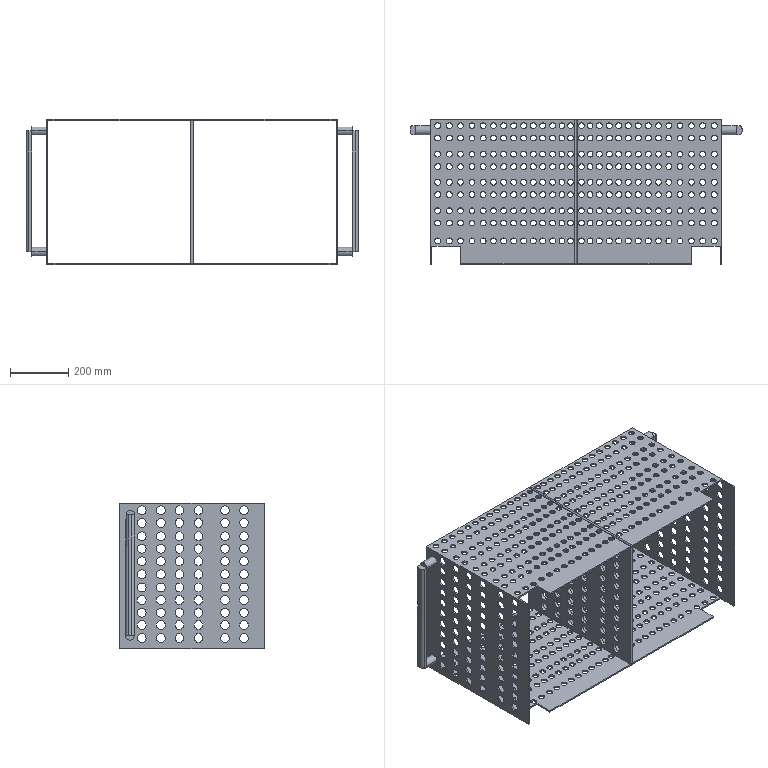Part | SolidWorks | features BaseBody 1 | 1 solid | 1462 faces | box 1140 x 495 x 500 mm | volume 8546977 mm3 | cylinder 1420 | plane 42 | commonest cylinder face diameters 20 x1012 30 x404 10 x4